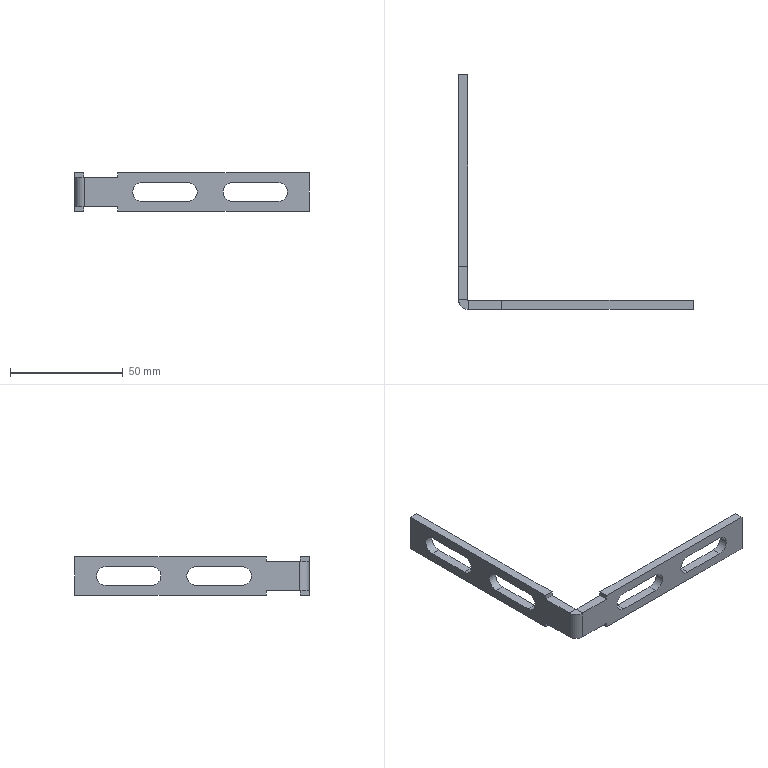Part | SolidWorks | features ICE 3, FlatPattern 1, SMBaseFlange 1, SheetMetal 1 | 1 solid | 40 faces | box 104 x 104 x 17 mm | volume 9651 mm3 | plane 28 | cylinder 12 | commonest cylinder face diameters 8.5 x10 0.4 x1 8.4 x1
STEP:
#1=CARTESIAN_POINT('',(4.,30.,12.75));
#2=VERTEX_POINT('',#1);
#3=CARTESIAN_POINT('',(4.,25.75,8.5));
#4=VERTEX_POINT('',#3);
#5=CARTESIAN_POINT('',(4.,30.,8.5));
#6=DIRECTION('',(1.,0.,0.));
#7=DIRECTION('',(0.,1.,0.));
#8=AXIS2_PLACEMENT_3D('',#5,#6,#7);
#9=CIRCLE('',#8,4.25);
#10=EDGE_CURVE('',#2,#4,#9,.T.);
#11=ORIENTED_EDGE('',*,*,#10,.T.);
#12=CARTESIAN_POINT('',(0.,25.75,8.5));
#13=VERTEX_POINT('',#12);
#14=CARTESIAN_POINT('',(10.,25.75,8.5));
#15=DIRECTION('',(-1.,0.,0.));
#16=VECTOR('',#15,1000.);
#17=LINE('',#14,#16);
#18=EDGE_CURVE('',#4,#13,#17,.T.);
#19=ORIENTED_EDGE('',*,*,#18,.T.);
#20=CARTESIAN_POINT('',(0.,30.,12.75));
#21=VERTEX_POINT('',#20);
#22=CARTESIAN_POINT('',(0.,30.,8.5));
#23=DIRECTION('',(-1.,0.,0.));
#24=DIRECTION('',(0.,-1.,0.));
#25=AXIS2_PLACEMENT_3D('',#22,#23,#24);
#26=CIRCLE('',#25,4.25);
#27=EDGE_CURVE('',#13,#21,#26,.T.);
#28=ORIENTED_EDGE('',*,*,#27,.T.);
#29=CARTESIAN_POINT('',(10.,30.,12.75));
#30=DIRECTION('',(-1.,0.,0.));
#31=VECTOR('',#30,1000.);
#32=LINE('',#29,#31);
#33=EDGE_CURVE('',#2,#21,#32,.T.);
#34=ORIENTED_EDGE('',*,*,#33,.F.);
#35=EDGE_LOOP('',(#11,#19,#28,#34));
#36=FACE_OUTER_BOUND('',#35,.T.);
#37=CARTESIAN_POINT('',(10.,30.,8.5));
#38=DIRECTION('',(-1.,0.,0.));
#39=DIRECTION('',(0.,-1.,0.));
#40=AXIS2_PLACEMENT_3D('',#37,#38,#39);
#41=CYLINDRICAL_SURFACE('',#40,4.25);
#42=ADVANCED_FACE('',(#36),#41,.F.);
#43=CARTESIAN_POINT('',(4.,70.,12.75));
#44=VERTEX_POINT('',#43);
#45=CARTESIAN_POINT('',(4.,65.75,8.5));
#46=VERTEX_POINT('',#45);
#47=CARTESIAN_POINT('',(4.,70.,8.5));
#48=DIRECTION('',(1.,0.,0.));
#49=DIRECTION('',(0.,1.,0.));
#50=AXIS2_PLACEMENT_3D('',#47,#48,#49);
#51=CIRCLE('',#50,4.25);
#52=EDGE_CURVE('',#44,#46,#51,.T.);
#53=ORIENTED_EDGE('',*,*,#52,.T.);
#54=CARTESIAN_POINT('',(0.,65.75,8.5));
#55=VERTEX_POINT('',#54);
#56=CARTESIAN_POINT('',(10.,65.75,8.5));
#57=DIRECTION('',(-1.,0.,0.));
#58=VECTOR('',#57,1000.);
#59=LINE('',#56,#58);
#60=EDGE_CURVE('',#46,#55,#59,.T.);
#61=ORIENTED_EDGE('',*,*,#60,.T.);
#62=CARTESIAN_POINT('',(0.,70.,12.75));
#63=VERTEX_POINT('',#62);
#64=CARTESIAN_POINT('',(0.,70.,8.5));
#65=DIRECTION('',(-1.,0.,0.));
#66=DIRECTION('',(0.,-1.,0.));
#67=AXIS2_PLACEMENT_3D('',#64,#65,#66);
#68=CIRCLE('',#67,4.25);
#69=EDGE_CURVE('',#55,#63,#68,.T.);
#70=ORIENTED_EDGE('',*,*,#69,.T.);
#71=CARTESIAN_POINT('',(10.,70.,12.75));
#72=DIRECTION('',(-1.,0.,0.));
#73=VECTOR('',#72,1000.);
#74=LINE('',#71,#73);
#75=EDGE_CURVE('',#44,#63,#74,.T.);
#76=ORIENTED_EDGE('',*,*,#75,.F.);
#77=EDGE_LOOP('',(#53,#61,#70,#76));
#78=FACE_OUTER_BOUND('',#77,.T.);
#79=CARTESIAN_POINT('',(10.,70.,8.5));
#80=DIRECTION('',(-1.,0.,0.));
#81=DIRECTION('',(0.,-1.,0.));
#82=AXIS2_PLACEMENT_3D('',#79,#80,#81);
#83=CYLINDRICAL_SURFACE('',#82,4.25);
#84=ADVANCED_FACE('',(#78),#83,.F.);
#85=CARTESIAN_POINT('',(0.,19.,15.));
#86=VERTEX_POINT('',#85);
#87=CARTESIAN_POINT('',(0.,4.2,15.));
#88=VERTEX_POINT('',#87);
#89=CARTESIAN_POINT('',(0.,0.,15.));
#90=DIRECTION('',(0.,-1.,0.));
#91=VECTOR('',#90,1000.);
#92=LINE('',#89,#91);
#93=EDGE_CURVE('',#86,#88,#92,.T.);
#94=ORIENTED_EDGE('',*,*,#93,.T.);
#95=CARTESIAN_POINT('',(4.,4.2,15.));
#96=VERTEX_POINT('',#95);
#97=CARTESIAN_POINT('',(0.,4.2,15.));
#98=DIRECTION('',(1.,0.,0.));
#99=VECTOR('',#98,1000.);
#100=LINE('',#97,#99);
#101=EDGE_CURVE('',#88,#96,#100,.T.);
#102=ORIENTED_EDGE('',*,*,#101,.T.);
#103=CARTESIAN_POINT('',(4.,19.,15.));
#104=VERTEX_POINT('',#103);
#105=CARTESIAN_POINT('',(4.,104.,15.));
#106=DIRECTION('',(0.,1.,0.));
#107=VECTOR('',#106,1000.);
#108=LINE('',#105,#107);
#109=EDGE_CURVE('',#96,#104,#108,.T.);
#110=ORIENTED_EDGE('',*,*,#109,.T.);
#111=CARTESIAN_POINT('',(19.,19.,15.));
#112=DIRECTION('',(-1.,0.,0.));
#113=VECTOR('',#112,1000.);
#114=LINE('',#111,#113);
#115=EDGE_CURVE('',#104,#86,#114,.T.);
#116=ORIENTED_EDGE('',*,*,#115,.T.);
#117=EDGE_LOOP('',(#94,#102,#110,#116));
#118=FACE_OUTER_BOUND('',#117,.T.);
#119=CARTESIAN_POINT('',(19.,0.,15.));
#120=DIRECTION('',(0.,0.,-1.));
#121=DIRECTION('',(-1.,0.,0.));
#122=AXIS2_PLACEMENT_3D('',#119,#120,#121);
#123=PLANE('',#122);
#124=ADVANCED_FACE('',(#118),#123,.F.);
#125=CARTESIAN_POINT('',(19.,4.,15.));
#126=VERTEX_POINT('',#125);
#127=CARTESIAN_POINT('',(4.2,4.,15.));
#128=VERTEX_POINT('',#127);
#129=CARTESIAN_POINT('',(0.,4.,15.));
#130=DIRECTION('',(-1.,0.,0.));
#131=VECTOR('',#130,1000.);
#132=LINE('',#129,#131);
#133=EDGE_CURVE('',#126,#128,#132,.T.);
#134=ORIENTED_EDGE('',*,*,#133,.T.);
#135=CARTESIAN_POINT('',(4.2,0.,15.));
#136=VERTEX_POINT('',#135);
#137=CARTESIAN_POINT('',(4.2,4.,15.));
#138=DIRECTION('',(0.,-1.,0.));
#139=VECTOR('',#138,1000.);
#140=LINE('',#137,#139);
#141=EDGE_CURVE('',#128,#136,#140,.T.);
#142=ORIENTED_EDGE('',*,*,#141,.T.);
#143=CARTESIAN_POINT('',(19.,0.,15.));
#144=VERTEX_POINT('',#143);
#145=CARTESIAN_POINT('',(19.,0.,15.));
#146=DIRECTION('',(-1.,0.,0.));
#147=VECTOR('',#146,1000.);
#148=LINE('',#145,#147);
#149=EDGE_CURVE('',#144,#136,#148,.T.);
#150=ORIENTED_EDGE('',*,*,#149,.F.);
#151=CARTESIAN_POINT('',(19.,0.,15.));
#152=DIRECTION('',(0.,-1.,0.));
#153=VECTOR('',#152,1000.);
#154=LINE('',#151,#153);
#155=EDGE_CURVE('',#126,#144,#154,.T.);
#156=ORIENTED_EDGE('',*,*,#155,.F.);
#157=EDGE_LOOP('',(#134,#142,#150,#156));
#158=FACE_OUTER_BOUND('',#157,.T.);
#159=CARTESIAN_POINT('',(19.,0.,15.));
#160=DIRECTION('',(0.,0.,-1.));
#161=DIRECTION('',(-1.,0.,0.));
#162=AXIS2_PLACEMENT_3D('',#159,#160,#161);
#163=PLANE('',#162);
#164=ADVANCED_FACE('',(#158),#163,.F.);
#165=CARTESIAN_POINT('',(4.,19.,2.));
#166=VERTEX_POINT('',#165);
#167=CARTESIAN_POINT('',(4.,4.2,2.));
#168=VERTEX_POINT('',#167);
#169=CARTESIAN_POINT('',(4.,104.,2.));
#170=DIRECTION('',(0.,-1.,0.));
#171=VECTOR('',#170,1000.);
#172=LINE('',#169,#171);
#173=EDGE_CURVE('',#166,#168,#172,.T.);
#174=ORIENTED_EDGE('',*,*,#173,.T.);
#175=CARTESIAN_POINT('',(0.,4.2,2.));
#176=VERTEX_POINT('',#175);
#177=CARTESIAN_POINT('',(4.,4.2,2.));
#178=DIRECTION('',(-1.,0.,0.));
#179=VECTOR('',#178,1000.);
#180=LINE('',#177,#179);
#181=EDGE_CURVE('',#168,#176,#180,.T.);
#182=ORIENTED_EDGE('',*,*,#181,.T.);
#183=CARTESIAN_POINT('',(0.,19.,2.));
#184=VERTEX_POINT('',#183);
#185=CARTESIAN_POINT('',(0.,0.,2.));
#186=DIRECTION('',(0.,1.,0.));
#187=VECTOR('',#186,1000.);
#188=LINE('',#185,#187);
#189=EDGE_CURVE('',#176,#184,#188,.T.);
#190=ORIENTED_EDGE('',*,*,#189,.T.);
#191=CARTESIAN_POINT('',(19.,19.,2.));
#192=DIRECTION('',(-1.,0.,0.));
#193=VECTOR('',#192,1000.);
#194=LINE('',#191,#193);
#195=EDGE_CURVE('',#166,#184,#194,.T.);
#196=ORIENTED_EDGE('',*,*,#195,.F.);
#197=EDGE_LOOP('',(#174,#182,#190,#196));
#198=FACE_OUTER_BOUND('',#197,.T.);
#199=CARTESIAN_POINT('',(19.,0.,2.));
#200=DIRECTION('',(0.,0.,1.));
#201=DIRECTION('',(1.,0.,0.));
#202=AXIS2_PLACEMENT_3D('',#199,#200,#201);
#203=PLANE('',#202);
#204=ADVANCED_FACE('',(#198),#203,.F.);
#205=CARTESIAN_POINT('',(19.,0.,2.));
#206=VERTEX_POINT('',#205);
#207=CARTESIAN_POINT('',(4.2,0.,2.));
#208=VERTEX_POINT('',#207);
#209=CARTESIAN_POINT('',(19.,0.,2.));
#210=DIRECTION('',(-1.,0.,0.));
#211=VECTOR('',#210,1000.);
#212=LINE('',#209,#211);
#213=EDGE_CURVE('',#206,#208,#212,.T.);
#214=ORIENTED_EDGE('',*,*,#213,.T.);
#215=CARTESIAN_POINT('',(4.2,4.,2.));
#216=VERTEX_POINT('',#215);
#217=CARTESIAN_POINT('',(4.2,0.,2.));
#218=DIRECTION('',(0.,1.,0.));
#219=VECTOR('',#218,1000.);
#220=LINE('',#217,#219);
#221=EDGE_CURVE('',#208,#216,#220,.T.);
#222=ORIENTED_EDGE('',*,*,#221,.T.);
#223=CARTESIAN_POINT('',(19.,4.,2.));
#224=VERTEX_POINT('',#223);
#225=CARTESIAN_POINT('',(0.,4.,2.));
#226=DIRECTION('',(1.,0.,0.));
#227=VECTOR('',#226,1000.);
#228=LINE('',#225,#227);
#229=EDGE_CURVE('',#216,#224,#228,.T.);
#230=ORIENTED_EDGE('',*,*,#229,.T.);
#231=CARTESIAN_POINT('',(19.,0.,2.));
#232=DIRECTION('',(0.,1.,0.));
#233=VECTOR('',#232,1000.);
#234=LINE('',#231,#233);
#235=EDGE_CURVE('',#206,#224,#234,.T.);
#236=ORIENTED_EDGE('',*,*,#235,.F.);
#237=EDGE_LOOP('',(#214,#222,#230,#236));
#238=FACE_OUTER_BOUND('',#237,.T.);
#239=CARTESIAN_POINT('',(19.,0.,2.));
#240=DIRECTION('',(0.,0.,1.));
#241=DIRECTION('',(1.,0.,0.));
#242=AXIS2_PLACEMENT_3D('',#239,#240,#241);
#243=PLANE('',#242);
#244=ADVANCED_FACE('',(#238),#243,.F.);
#245=CARTESIAN_POINT('',(19.,0.,0.));
#246=VERTEX_POINT('',#245);
#247=CARTESIAN_POINT('',(104.,0.,0.));
#248=VERTEX_POINT('',#247);
#249=CARTESIAN_POINT('',(0.,0.,0.));
#250=DIRECTION('',(1.,0.,0.));
#251=VECTOR('',#250,1000.);
#252=LINE('',#249,#251);
#253=EDGE_CURVE('',#246,#248,#252,.T.);
#254=ORIENTED_EDGE('',*,*,#253,.F.);
#255=CARTESIAN_POINT('',(19.,4.,0.));
#256=VERTEX_POINT('',#255);
#257=CARTESIAN_POINT('',(19.,0.,0.));
#258=DIRECTION('',(0.,-1.,0.));
#259=VECTOR('',#258,1000.);
#260=LINE('',#257,#259);
#261=EDGE_CURVE('',#256,#246,#260,.T.);
#262=ORIENTED_EDGE('',*,*,#261,.F.);
#263=CARTESIAN_POINT('',(104.,4.,0.));
#264=VERTEX_POINT('',#263);
#265=CARTESIAN_POINT('',(0.,4.,0.));
#266=DIRECTION('',(1.,0.,0.));
#267=VECTOR('',#266,1000.);
#268=LINE('',#265,#267);
#269=EDGE_CURVE('',#256,#264,#268,.T.);
#270=ORIENTED_EDGE('',*,*,#269,.T.);
#271=CARTESIAN_POINT('',(104.,4.,0.));
#272=DIRECTION('',(0.,-1.,0.));
#273=VECTOR('',#272,1000.);
#274=LINE('',#271,#273);
#275=EDGE_CURVE('',#264,#248,#274,.T.);
#276=ORIENTED_EDGE('',*,*,#275,.T.);
#277=EDGE_LOOP('',(#254,#262,#270,#276));
#278=FACE_OUTER_BOUND('',#277,.T.);
#279=CARTESIAN_POINT('',(4.,4.2,0.));
#280=DIRECTION('',(0.,0.,-1.));
#281=DIRECTION('',(-1.,0.,0.));
#282=AXIS2_PLACEMENT_3D('',#279,#280,#281);
#283=PLANE('',#282);
#284=ADVANCED_FACE('',(#278),#283,.T.);
#285=CARTESIAN_POINT('',(19.,4.,17.));
#286=VERTEX_POINT('',#285);
#287=CARTESIAN_POINT('',(104.,4.,17.));
#288=VERTEX_POINT('',#287);
#289=CARTESIAN_POINT('',(0.,4.,17.));
#290=DIRECTION('',(1.,0.,0.));
#291=VECTOR('',#290,1000.);
#292=LINE('',#289,#291);
#293=EDGE_CURVE('',#286,#288,#292,.T.);
#294=ORIENTED_EDGE('',*,*,#293,.F.);
#295=CARTESIAN_POINT('',(19.,0.,17.));
#296=VERTEX_POINT('',#295);
#297=CARTESIAN_POINT('',(19.,0.,17.));
#298=DIRECTION('',(0.,1.,0.));
#299=VECTOR('',#298,1000.);
#300=LINE('',#297,#299);
#301=EDGE_CURVE('',#296,#286,#300,.T.);
#302=ORIENTED_EDGE('',*,*,#301,.F.);
#303=CARTESIAN_POINT('',(104.,0.,17.));
#304=VERTEX_POINT('',#303);
#305=CARTESIAN_POINT('',(0.,0.,17.));
#306=DIRECTION('',(1.,0.,0.));
#307=VECTOR('',#306,1000.);
#308=LINE('',#305,#307);
#309=EDGE_CURVE('',#296,#304,#308,.T.);
#310=ORIENTED_EDGE('',*,*,#309,.T.);
#311=CARTESIAN_POINT('',(104.,4.,17.));
#312=DIRECTION('',(0.,-1.,0.));
#313=VECTOR('',#312,1000.);
#314=LINE('',#311,#313);
#315=EDGE_CURVE('',#288,#304,#314,.T.);
#316=ORIENTED_EDGE('',*,*,#315,.F.);
#317=EDGE_LOOP('',(#294,#302,#310,#316));
#318=FACE_OUTER_BOUND('',#317,.T.);
#319=CARTESIAN_POINT('',(4.2,4.2,17.));
#320=DIRECTION('',(0.,0.,1.));
#321=DIRECTION('',(1.,0.,0.));
#322=AXIS2_PLACEMENT_3D('',#319,#320,#321);
#323=PLANE('',#322);
#324=ADVANCED_FACE('',(#318),#323,.T.);
#325=CARTESIAN_POINT('',(4.,19.,17.));
#326=VERTEX_POINT('',#325);
#327=CARTESIAN_POINT('',(0.,19.,17.));
#328=VERTEX_POINT('',#327);
#329=CARTESIAN_POINT('',(19.,19.,17.));
#330=DIRECTION('',(-1.,0.,0.));
#331=VECTOR('',#330,1000.);
#332=LINE('',#329,#331);
#333=EDGE_CURVE('',#326,#328,#332,.T.);
#334=ORIENTED_EDGE('',*,*,#333,.F.);
#335=CARTESIAN_POINT('',(4.,104.,17.));
#336=VERTEX_POINT('',#335);
#337=CARTESIAN_POINT('',(4.,104.,17.));
#338=DIRECTION('',(0.,-1.,0.));
#339=VECTOR('',#338,1000.);
#340=LINE('',#337,#339);
#341=EDGE_CURVE('',#336,#326,#340,.T.);
#342=ORIENTED_EDGE('',*,*,#341,.F.);
#343=CARTESIAN_POINT('',(0.,104.,17.));
#344=VERTEX_POINT('',#343);
#345=CARTESIAN_POINT('',(0.,104.,17.));
#346=DIRECTION('',(1.,0.,0.));
#347=VECTOR('',#346,1000.);
#348=LINE('',#345,#347);
#349=EDGE_CURVE('',#344,#336,#348,.T.);
#350=ORIENTED_EDGE('',*,*,#349,.F.);
#351=CARTESIAN_POINT('',(0.,104.,17.));
#352=DIRECTION('',(0.,-1.,0.));
#353=VECTOR('',#352,1000.);
#354=LINE('',#351,#353);
#355=EDGE_CURVE('',#344,#328,#354,.T.);
#356=ORIENTED_EDGE('',*,*,#355,.T.);
#357=EDGE_LOOP('',(#334,#342,#350,#356));
#358=FACE_OUTER_BOUND('',#357,.T.);
#359=CARTESIAN_POINT('',(4.2,4.,17.));
#360=DIRECTION('',(0.,0.,1.));
#361=DIRECTION('',(1.,0.,0.));
#362=AXIS2_PLACEMENT_3D('',#359,#360,#361);
#363=PLANE('',#362);
#364=ADVANCED_FACE('',(#358),#363,.T.);
#365=CARTESIAN_POINT('',(30.,0.,4.25));
#366=VERTEX_POINT('',#365);
#367=CARTESIAN_POINT('',(50.,0.,4.25));
#368=VERTEX_POINT('',#367);
#369=CARTESIAN_POINT('',(30.,0.,4.25));
#370=DIRECTION('',(1.,0.,0.));
#371=VECTOR('',#370,1000.);
#372=LINE('',#369,#371);
#373=EDGE_CURVE('',#366,#368,#372,.T.);
#374=ORIENTED_EDGE('',*,*,#373,.F.);
#375=CARTESIAN_POINT('',(30.,0.,12.75));
#376=VERTEX_POINT('',#375);
#377=CARTESIAN_POINT('',(30.,0.,8.5));
#378=DIRECTION('',(0.,-1.,0.));
#379=DIRECTION('',(0.,0.,-1.));
#380=AXIS2_PLACEMENT_3D('',#377,#378,#379);
#381=CIRCLE('',#380,4.25);
#382=EDGE_CURVE('',#376,#366,#381,.T.);
#383=ORIENTED_EDGE('',*,*,#382,.F.);
#384=CARTESIAN_POINT('',(50.,0.,12.75));
#385=VERTEX_POINT('',#384);
#386=CARTESIAN_POINT('',(30.,0.,12.75));
#387=DIRECTION('',(-1.,0.,0.));
#388=VECTOR('',#387,1000.);
#389=LINE('',#386,#388);
#390=EDGE_CURVE('',#385,#376,#389,.T.);
#391=ORIENTED_EDGE('',*,*,#390,.F.);
#392=CARTESIAN_POINT('',(50.,0.,8.5));
#393=DIRECTION('',(0.,-1.,0.));
#394=DIRECTION('',(0.,0.,-1.));
#395=AXIS2_PLACEMENT_3D('',#392,#393,#394);
#396=CIRCLE('',#395,4.25);
#397=EDGE_CURVE('',#368,#385,#396,.T.);
#398=ORIENTED_EDGE('',*,*,#397,.F.);
#399=EDGE_LOOP('',(#374,#383,#391,#398));
#400=FACE_BOUND('',#399,.T.);
#401=CARTESIAN_POINT('',(70.,0.,4.25));
#402=VERTEX_POINT('',#401);
#403=CARTESIAN_POINT('',(90.,0.,4.25));
#404=VERTEX_POINT('',#403);
#405=CARTESIAN_POINT('',(70.,0.,4.25));
#406=DIRECTION('',(1.,0.,0.));
#407=VECTOR('',#406,1000.);
#408=LINE('',#405,#407);
#409=EDGE_CURVE('',#402,#404,#408,.T.);
#410=ORIENTED_EDGE('',*,*,#409,.F.);
#411=CARTESIAN_POINT('',(70.,0.,12.75));
#412=VERTEX_POINT('',#411);
#413=CARTESIAN_POINT('',(70.,0.,8.5));
#414=DIRECTION('',(0.,-1.,0.));
#415=DIRECTION('',(0.,0.,-1.));
#416=AXIS2_PLACEMENT_3D('',#413,#414,#415);
#417=CIRCLE('',#416,4.25);
#418=EDGE_CURVE('',#412,#402,#417,.T.);
#419=ORIENTED_EDGE('',*,*,#418,.F.);
#420=CARTESIAN_POINT('',(90.,0.,12.75));
#421=VERTEX_POINT('',#420);
#422=CARTESIAN_POINT('',(70.,0.,12.75));
#423=DIRECTION('',(-1.,0.,0.));
#424=VECTOR('',#423,1000.);
#425=LINE('',#422,#424);
#426=EDGE_CURVE('',#421,#412,#425,.T.);
#427=ORIENTED_EDGE('',*,*,#426,.F.);
#428=CARTESIAN_POINT('',(90.,0.,8.5));
#429=DIRECTION('',(0.,-1.,0.));
#430=DIRECTION('',(0.,0.,-1.));
#431=AXIS2_PLACEMENT_3D('',#428,#429,#430);
#432=CIRCLE('',#431,4.25);
#433=EDGE_CURVE('',#404,#421,#432,.T.);
#434=ORIENTED_EDGE('',*,*,#433,.F.);
#435=EDGE_LOOP('',(#410,#419,#427,#434));
#436=FACE_BOUND('',#435,.T.);
#437=CARTESIAN_POINT('',(19.,0.,17.));
#438=DIRECTION('',(0.,0.,1.));
#439=VECTOR('',#438,1000.);
#440=LINE('',#437,#439);
#441=EDGE_CURVE('',#144,#296,#440,.T.);
#442=ORIENTED_EDGE('',*,*,#441,.F.);
#443=ORIENTED_EDGE('',*,*,#149,.T.);
#444=CARTESIAN_POINT('',(4.2,0.,17.));
#445=DIRECTION('',(0.,0.,-1.));
#446=VECTOR('',#445,1000.);
#447=LINE('',#444,#446);
#448=EDGE_CURVE('',#136,#208,#447,.T.);
#449=ORIENTED_EDGE('',*,*,#448,.T.);
#450=ORIENTED_EDGE('',*,*,#213,.F.);
#451=CARTESIAN_POINT('',(19.,0.,0.));
#452=DIRECTION('',(0.,0.,1.));
#453=VECTOR('',#452,1000.);
#454=LINE('',#451,#453);
#455=EDGE_CURVE('',#246,#206,#454,.T.);
#456=ORIENTED_EDGE('',*,*,#455,.F.);
#457=ORIENTED_EDGE('',*,*,#253,.T.);
#458=CARTESIAN_POINT('',(104.,0.,17.));
#459=DIRECTION('',(0.,0.,-1.));
#460=VECTOR('',#459,1000.);
#461=LINE('',#458,#460);
#462=EDGE_CURVE('',#304,#248,#461,.T.);
#463=ORIENTED_EDGE('',*,*,#462,.F.);
#464=ORIENTED_EDGE('',*,*,#309,.F.);
#465=EDGE_LOOP('',(#442,#443,#449,#450,#456,#457,#463,#464));
#466=FACE_OUTER_BOUND('',#465,.T.);
#467=CARTESIAN_POINT('',(0.,0.,17.));
#468=DIRECTION('',(0.,1.,0.));
#469=DIRECTION('',(0.,0.,1.));
#470=AXIS2_PLACEMENT_3D('',#467,#468,#469);
#471=PLANE('',#470);
#472=ADVANCED_FACE('',(#400,#436,#466),#471,.F.);
#473=ORIENTED_EDGE('',*,*,#275,.F.);
#474=CARTESIAN_POINT('',(104.,4.,17.));
#475=DIRECTION('',(0.,0.,-1.));
#476=VECTOR('',#475,1000.);
#477=LINE('',#474,#476);
#478=EDGE_CURVE('',#288,#264,#477,.T.);
#479=ORIENTED_EDGE('',*,*,#478,.F.);
#480=ORIENTED_EDGE('',*,*,#315,.T.);
#481=ORIENTED_EDGE('',*,*,#462,.T.);
#482=EDGE_LOOP('',(#473,#479,#480,#481));
#483=FACE_OUTER_BOUND('',#482,.T.);
#484=CARTESIAN_POINT('',(104.,4.,17.));
#485=DIRECTION('',(1.,0.,0.));
#486=DIRECTION('',(0.,0.,-1.));
#487=AXIS2_PLACEMENT_3D('',#484,#485,#486);
#488=PLANE('',#487);
#489=ADVANCED_FACE('',(#483),#488,.T.);
#490=ORIENTED_EDGE('',*,*,#133,.F.);
#491=CARTESIAN_POINT('',(19.,4.,17.));
#492=DIRECTION('',(0.,0.,1.));
#493=VECTOR('',#492,1000.);
#494=LINE('',#491,#493);
#495=EDGE_CURVE('',#126,#286,#494,.T.);
#496=ORIENTED_EDGE('',*,*,#495,.T.);
#497=ORIENTED_EDGE('',*,*,#293,.T.);
#498=ORIENTED_EDGE('',*,*,#478,.T.);
#499=ORIENTED_EDGE('',*,*,#269,.F.);
#500=CARTESIAN_POINT('',(19.,4.,17.));
#501=DIRECTION('',(0.,0.,1.));
#502=VECTOR('',#501,1000.);
#503=LINE('',#500,#502);
#504=EDGE_CURVE('',#256,#224,#503,.T.);
#505=ORIENTED_EDGE('',*,*,#504,.T.);
#506=ORIENTED_EDGE('',*,*,#229,.F.);
#507=CARTESIAN_POINT('',(4.2,4.,17.));
#508=DIRECTION('',(0.,0.,-1.));
#509=VECTOR('',#508,1000.);
#510=LINE('',#507,#509);
#511=EDGE_CURVE('',#128,#216,#510,.T.);
#512=ORIENTED_EDGE('',*,*,#511,.F.);
#513=EDGE_LOOP('',(#490,#496,#497,#498,#499,#505,#506,#512));
#514=FACE_OUTER_BOUND('',#513,.T.);
#515=CARTESIAN_POINT('',(30.,4.,4.25));
#516=VERTEX_POINT('',#515);
#517=CARTESIAN_POINT('',(30.,4.,12.75));
#518=VERTEX_POINT('',#517);
#519=CARTESIAN_POINT('',(30.,4.,8.5));
#520=DIRECTION('',(0.,1.,0.));
#521=DIRECTION('',(0.,0.,1.));
#522=AXIS2_PLACEMENT_3D('',#519,#520,#521);
#523=CIRCLE('',#522,4.25);
#524=EDGE_CURVE('',#516,#518,#523,.T.);
#525=ORIENTED_EDGE('',*,*,#524,.F.);
#526=CARTESIAN_POINT('',(50.,4.,4.25));
#527=VERTEX_POINT('',#526);
#528=CARTESIAN_POINT('',(0.,4.,4.25));
#529=DIRECTION('',(-1.,0.,0.));
#530=VECTOR('',#529,1000.);
#531=LINE('',#528,#530);
#532=EDGE_CURVE('',#527,#516,#531,.T.);
#533=ORIENTED_EDGE('',*,*,#532,.F.);
#534=CARTESIAN_POINT('',(50.,4.,12.75));
#535=VERTEX_POINT('',#534);
#536=CARTESIAN_POINT('',(50.,4.,8.5));
#537=DIRECTION('',(0.,1.,0.));
#538=DIRECTION('',(0.,0.,1.));
#539=AXIS2_PLACEMENT_3D('',#536,#537,#538);
#540=CIRCLE('',#539,4.25);
#541=EDGE_CURVE('',#535,#527,#540,.T.);
#542=ORIENTED_EDGE('',*,*,#541,.F.);
#543=CARTESIAN_POINT('',(0.,4.,12.75));
#544=DIRECTION('',(1.,0.,0.));
#545=VECTOR('',#544,1000.);
#546=LINE('',#543,#545);
#547=EDGE_CURVE('',#518,#535,#546,.T.);
#548=ORIENTED_EDGE('',*,*,#547,.F.);
#549=EDGE_LOOP('',(#525,#533,#542,#548));
#550=FACE_BOUND('',#549,.T.);
#551=CARTESIAN_POINT('',(70.,4.,4.25));
#552=VERTEX_POINT('',#551);
#553=CARTESIAN_POINT('',(70.,4.,12.75));
#554=VERTEX_POINT('',#553);
#555=CARTESIAN_POINT('',(70.,4.,8.5));
#556=DIRECTION('',(0.,1.,0.));
#557=DIRECTION('',(0.,0.,1.));
#558=AXIS2_PLACEMENT_3D('',#555,#556,#557);
#559=CIRCLE('',#558,4.25);
#560=EDGE_CURVE('',#552,#554,#559,.T.);
#561=ORIENTED_EDGE('',*,*,#560,.F.);
#562=CARTESIAN_POINT('',(90.,4.,4.25));
#563=VERTEX_POINT('',#562);
#564=CARTESIAN_POINT('',(0.,4.,4.25));
#565=DIRECTION('',(-1.,0.,0.));
#566=VECTOR('',#565,1000.);
#567=LINE('',#564,#566);
#568=EDGE_CURVE('',#563,#552,#567,.T.);
#569=ORIENTED_EDGE('',*,*,#568,.F.);
#570=CARTESIAN_POINT('',(90.,4.,12.75));
#571=VERTEX_POINT('',#570);
#572=CARTESIAN_POINT('',(90.,4.,8.5));
#573=DIRECTION('',(0.,1.,0.));
#574=DIRECTION('',(0.,0.,1.));
#575=AXIS2_PLACEMENT_3D('',#572,#573,#574);
#576=CIRCLE('',#575,4.25);
#577=EDGE_CURVE('',#571,#563,#576,.T.);
#578=ORIENTED_EDGE('',*,*,#577,.F.);
#579=CARTESIAN_POINT('',(0.,4.,12.75));
#580=DIRECTION('',(1.,0.,0.));
#581=VECTOR('',#580,1000.);
#582=LINE('',#579,#581);
#583=EDGE_CURVE('',#554,#571,#582,.T.);
#584=ORIENTED_EDGE('',*,*,#583,.F.);
#585=EDGE_LOOP('',(#561,#569,#578,#584));
#586=FACE_BOUND('',#585,.T.);
#587=CARTESIAN_POINT('',(0.,4.,17.));
#588=DIRECTION('',(0.,1.,0.));
#589=DIRECTION('',(0.,0.,1.));
#590=AXIS2_PLACEMENT_3D('',#587,#588,#589);
#591=PLANE('',#590);
#592=ADVANCED_FACE('',(#514,#550,#586),#591,.T.);
#593=CARTESIAN_POINT('',(4.2,4.2,15.));
#594=DIRECTION('',(0.,0.,-1.));
#595=DIRECTION('',(-1.,0.,0.));
#596=AXIS2_PLACEMENT_3D('',#593,#594,#595);
#597=CIRCLE('',#596,0.2);
#598=EDGE_CURVE('',#128,#96,#597,.T.);
#599=ORIENTED_EDGE('',*,*,#598,.F.);
#600=ORIENTED_EDGE('',*,*,#511,.T.);
#601=CARTESIAN_POINT('',(4.2,4.2,2.));
#602=DIRECTION('',(0.,0.,1.));
#603=DIRECTION('',(1.,0.,0.));
#604=AXIS2_PLACEMENT_3D('',#601,#602,#603);
#605=CIRCLE('',#604,0.2);
#606=EDGE_CURVE('',#168,#216,#605,.T.);
#607=ORIENTED_EDGE('',*,*,#606,.F.);
#608=CARTESIAN_POINT('',(4.,4.2,17.));
#609=DIRECTION('',(0.,0.,-1.));
#610=VECTOR('',#609,1000.);
#611=LINE('',#608,#610);
#612=EDGE_CURVE('',#96,#168,#611,.T.);
#613=ORIENTED_EDGE('',*,*,#612,.F.);
#614=EDGE_LOOP('',(#599,#600,#607,#613));
#615=FACE_OUTER_BOUND('',#614,.T.);
#616=CARTESIAN_POINT('',(4.2,4.2,17.));
#617=DIRECTION('',(0.,0.,-1.));
#618=DIRECTION('',(-1.,0.,0.));
#619=AXIS2_PLACEMENT_3D('',#616,#617,#618);
#620=CYLINDRICAL_SURFACE('',#619,0.2);
#621=ADVANCED_FACE('',(#615),#620,.F.);
#622=ORIENTED_EDGE('',*,*,#109,.F.);
#623=ORIENTED_EDGE('',*,*,#612,.T.);
#624=ORIENTED_EDGE('',*,*,#173,.F.);
#625=CARTESIAN_POINT('',(4.,19.,0.));
#626=VERTEX_POINT('',#625);
#627=CARTESIAN_POINT('',(4.,19.,17.));
#628=DIRECTION('',(0.,0.,1.));
#629=VECTOR('',#628,1000.);
#630=LINE('',#627,#629);
#631=EDGE_CURVE('',#626,#166,#630,.T.);
#632=ORIENTED_EDGE('',*,*,#631,.F.);
#633=CARTESIAN_POINT('',(4.,104.,0.));
#634=VERTEX_POINT('',#633);
#635=CARTESIAN_POINT('',(4.,104.,0.));
#636=DIRECTION('',(0.,-1.,0.));
#637=VECTOR('',#636,1000.);
#638=LINE('',#635,#637);
#639=EDGE_CURVE('',#634,#626,#638,.T.);
#640=ORIENTED_EDGE('',*,*,#639,.F.);
#641=CARTESIAN_POINT('',(4.,104.,17.));
#642=DIRECTION('',(0.,0.,-1.));
#643=VECTOR('',#642,1000.);
#644=LINE('',#641,#643);
#645=EDGE_CURVE('',#336,#634,#644,.T.);
#646=ORIENTED_EDGE('',*,*,#645,.F.);
#647=ORIENTED_EDGE('',*,*,#341,.T.);
#648=CARTESIAN_POINT('',(4.,19.,17.));
#649=DIRECTION('',(0.,0.,1.));
#650=VECTOR('',#649,1000.);
#651=LINE('',#648,#650);
#652=EDGE_CURVE('',#104,#326,#651,.T.);
#653=ORIENTED_EDGE('',*,*,#652,.F.);
#654=EDGE_LOOP('',(#622,#623,#624,#632,#640,#646,#647,#653));
#655=FACE_OUTER_BOUND('',#654,.T.);
#656=CARTESIAN_POINT('',(4.,50.,4.25));
#657=VERTEX_POINT('',#656);
#658=CARTESIAN_POINT('',(4.,50.,12.75));
#659=VERTEX_POINT('',#658);
#660=CARTESIAN_POINT('',(4.,50.,8.5));
#661=DIRECTION('',(1.,0.,0.));
#662=DIRECTION('',(0.,1.,0.));
#663=AXIS2_PLACEMENT_3D('',#660,#661,#662);
#664=CIRCLE('',#663,4.25);
#665=EDGE_CURVE('',#657,#659,#664,.T.);
#666=ORIENTED_EDGE('',*,*,#665,.F.);
#667=CARTESIAN_POINT('',(4.,30.,4.25));
#668=VERTEX_POINT('',#667);
#669=CARTESIAN_POINT('',(4.,104.,4.25));
#670=DIRECTION('',(0.,1.,0.));
#671=VECTOR('',#670,1000.);
#672=LINE('',#669,#671);
#673=EDGE_CURVE('',#668,#657,#672,.T.);
#674=ORIENTED_EDGE('',*,*,#673,.F.);
#675=CARTESIAN_POINT('',(4.,30.,8.5));
#676=DIRECTION('',(1.,0.,0.));
#677=DIRECTION('',(0.,1.,0.));
#678=AXIS2_PLACEMENT_3D('',#675,#676,#677);
#679=CIRCLE('',#678,4.25);
#680=EDGE_CURVE('',#4,#668,#679,.T.);
#681=ORIENTED_EDGE('',*,*,#680,.F.);
#682=ORIENTED_EDGE('',*,*,#10,.F.);
#683=CARTESIAN_POINT('',(4.,104.,12.75));
#684=DIRECTION('',(0.,-1.,0.));
#685=VECTOR('',#684,1000.);
#686=LINE('',#683,#685);
#687=EDGE_CURVE('',#659,#2,#686,.T.);
#688=ORIENTED_EDGE('',*,*,#687,.F.);
#689=EDGE_LOOP('',(#666,#674,#681,#682,#688));
#690=FACE_BOUND('',#689,.T.);
#691=CARTESIAN_POINT('',(4.,90.,4.25));
#692=VERTEX_POINT('',#691);
#693=CARTESIAN_POINT('',(4.,90.,12.75));
#694=VERTEX_POINT('',#693);
#695=CARTESIAN_POINT('',(4.,90.,8.5));
#696=DIRECTION('',(1.,0.,0.));
#697=DIRECTION('',(0.,1.,0.));
#698=AXIS2_PLACEMENT_3D('',#695,#696,#697);
#699=CIRCLE('',#698,4.25);
#700=EDGE_CURVE('',#692,#694,#699,.T.);
#701=ORIENTED_EDGE('',*,*,#700,.F.);
#702=CARTESIAN_POINT('',(4.,70.,4.25));
#703=VERTEX_POINT('',#702);
#704=CARTESIAN_POINT('',(4.,104.,4.25));
#705=DIRECTION('',(0.,1.,0.));
#706=VECTOR('',#705,1000.);
#707=LINE('',#704,#706);
#708=EDGE_CURVE('',#703,#692,#707,.T.);
#709=ORIENTED_EDGE('',*,*,#708,.F.);
#710=CARTESIAN_POINT('',(4.,70.,8.5));
#711=DIRECTION('',(1.,0.,0.));
#712=DIRECTION('',(0.,1.,0.));
#713=AXIS2_PLACEMENT_3D('',#710,#711,#712);
#714=CIRCLE('',#713,4.25);
#715=EDGE_CURVE('',#46,#703,#714,.T.);
#716=ORIENTED_EDGE('',*,*,#715,.F.);
#717=ORIENTED_EDGE('',*,*,#52,.F.);
#718=CARTESIAN_POINT('',(4.,104.,12.75));
#719=DIRECTION('',(0.,-1.,0.));
#720=VECTOR('',#719,1000.);
#721=LINE('',#718,#720);
#722=EDGE_CURVE('',#694,#44,#721,.T.);
#723=ORIENTED_EDGE('',*,*,#722,.F.);
#724=EDGE_LOOP('',(#701,#709,#716,#717,#723));
#725=FACE_BOUND('',#724,.T.);
#726=CARTESIAN_POINT('',(4.,104.,17.));
#727=DIRECTION('',(1.,0.,0.));
#728=DIRECTION('',(0.,1.,0.));
#729=AXIS2_PLACEMENT_3D('',#726,#727,#728);
#730=PLANE('',#729);
#731=ADVANCED_FACE('',(#655,#690,#725),#730,.T.);
#732=CARTESIAN_POINT('',(0.,104.,0.));
#733=VERTEX_POINT('',#732);
#734=CARTESIAN_POINT('',(0.,104.,0.));
#735=DIRECTION('',(1.,0.,0.));
#736=VECTOR('',#735,1000.);
#737=LINE('',#734,#736);
#738=EDGE_CURVE('',#733,#634,#737,.T.);
#739=ORIENTED_EDGE('',*,*,#738,.F.);
#740=CARTESIAN_POINT('',(0.,104.,17.));
#741=DIRECTION('',(0.,0.,-1.));
#742=VECTOR('',#741,1000.);
#743=LINE('',#740,#742);
#744=EDGE_CURVE('',#344,#733,#743,.T.);
#745=ORIENTED_EDGE('',*,*,#744,.F.);
#746=ORIENTED_EDGE('',*,*,#349,.T.);
#747=ORIENTED_EDGE('',*,*,#645,.T.);
#748=EDGE_LOOP('',(#739,#745,#746,#747));
#749=FACE_OUTER_BOUND('',#748,.T.);
#750=CARTESIAN_POINT('',(0.,104.,17.));
#751=DIRECTION('',(0.,1.,0.));
#752=DIRECTION('',(0.,0.,1.));
#753=AXIS2_PLACEMENT_3D('',#750,#751,#752);
#754=PLANE('',#753);
#755=ADVANCED_FACE('',(#749),#754,.T.);
#756=CARTESIAN_POINT('',(0.,50.,4.25));
#757=VERTEX_POINT('',#756);
#758=CARTESIAN_POINT('',(0.,30.,4.25));
#759=VERTEX_POINT('',#758);
#760=CARTESIAN_POINT('',(0.,50.,4.25));
#761=DIRECTION('',(0.,-1.,0.));
#762=VECTOR('',#761,1000.);
#763=LINE('',#760,#762);
#764=EDGE_CURVE('',#757,#759,#763,.T.);
#765=ORIENTED_EDGE('',*,*,#764,.F.);
#766=CARTESIAN_POINT('',(0.,50.,12.75));
#767=VERTEX_POINT('',#766);
#768=CARTESIAN_POINT('',(0.,50.,8.5));
#769=DIRECTION('',(-1.,0.,0.));
#770=DIRECTION('',(0.,-1.,0.));
#771=AXIS2_PLACEMENT_3D('',#768,#769,#770);
#772=CIRCLE('',#771,4.25);
#773=EDGE_CURVE('',#767,#757,#772,.T.);
#774=ORIENTED_EDGE('',*,*,#773,.F.);
#775=CARTESIAN_POINT('',(0.,50.,12.75));
#776=DIRECTION('',(0.,1.,0.));
#777=VECTOR('',#776,1000.);
#778=LINE('',#775,#777);
#779=EDGE_CURVE('',#21,#767,#778,.T.);
#780=ORIENTED_EDGE('',*,*,#779,.F.);
#781=ORIENTED_EDGE('',*,*,#27,.F.);
#782=CARTESIAN_POINT('',(0.,30.,8.5));
#783=DIRECTION('',(-1.,0.,0.));
#784=DIRECTION('',(0.,-1.,0.));
#785=AXIS2_PLACEMENT_3D('',#782,#783,#784);
#786=CIRCLE('',#785,4.25);
#787=EDGE_CURVE('',#759,#13,#786,.T.);
#788=ORIENTED_EDGE('',*,*,#787,.F.);
#789=EDGE_LOOP('',(#765,#774,#780,#781,#788));
#790=FACE_BOUND('',#789,.T.);
#791=CARTESIAN_POINT('',(0.,90.,4.25));
#792=VERTEX_POINT('',#791);
#793=CARTESIAN_POINT('',(0.,70.,4.25));
#794=VERTEX_POINT('',#793);
#795=CARTESIAN_POINT('',(0.,90.,4.25));
#796=DIRECTION('',(0.,-1.,0.));
#797=VECTOR('',#796,1000.);
#798=LINE('',#795,#797);
#799=EDGE_CURVE('',#792,#794,#798,.T.);
#800=ORIENTED_EDGE('',*,*,#799,.F.);
#801=CARTESIAN_POINT('',(0.,90.,12.75));
#802=VERTEX_POINT('',#801);
#803=CARTESIAN_POINT('',(0.,90.,8.5));
#804=DIRECTION('',(-1.,0.,0.));
#805=DIRECTION('',(0.,-1.,0.));
#806=AXIS2_PLACEMENT_3D('',#803,#804,#805);
#807=CIRCLE('',#806,4.25);
#808=EDGE_CURVE('',#802,#792,#807,.T.);
#809=ORIENTED_EDGE('',*,*,#808,.F.);
#810=CARTESIAN_POINT('',(0.,90.,12.75));
#811=DIRECTION('',(0.,1.,0.));
#812=VECTOR('',#811,1000.);
#813=LINE('',#810,#812);
#814=EDGE_CURVE('',#63,#802,#813,.T.);
#815=ORIENTED_EDGE('',*,*,#814,.F.);
#816=ORIENTED_EDGE('',*,*,#69,.F.);
#817=CARTESIAN_POINT('',(0.,70.,8.5));
#818=DIRECTION('',(-1.,0.,0.));
#819=DIRECTION('',(0.,-1.,0.));
#820=AXIS2_PLACEMENT_3D('',#817,#818,#819);
#821=CIRCLE('',#820,4.25);
#822=EDGE_CURVE('',#794,#55,#821,.T.);
#823=ORIENTED_EDGE('',*,*,#822,.F.);
#824=EDGE_LOOP('',(#800,#809,#815,#816,#823));
#825=FACE_BOUND('',#824,.T.);
#826=CARTESIAN_POINT('',(0.,4.2,17.));
#827=DIRECTION('',(0.,0.,-1.));
#828=VECTOR('',#827,1000.);
#829=LINE('',#826,#828);
#830=EDGE_CURVE('',#88,#176,#829,.T.);
#831=ORIENTED_EDGE('',*,*,#830,.F.);
#832=ORIENTED_EDGE('',*,*,#93,.F.);
#833=CARTESIAN_POINT('',(0.,19.,17.));
#834=DIRECTION('',(0.,0.,-1.));
#835=VECTOR('',#834,1000.);
#836=LINE('',#833,#835);
#837=EDGE_CURVE('',#328,#86,#836,.T.);
#838=ORIENTED_EDGE('',*,*,#837,.F.);
#839=ORIENTED_EDGE('',*,*,#355,.F.);
#840=ORIENTED_EDGE('',*,*,#744,.T.);
#841=CARTESIAN_POINT('',(0.,19.,0.));
#842=VERTEX_POINT('',#841);
#843=CARTESIAN_POINT('',(0.,104.,0.));
#844=DIRECTION('',(0.,-1.,0.));
#845=VECTOR('',#844,1000.);
#846=LINE('',#843,#845);
#847=EDGE_CURVE('',#733,#842,#846,.T.);
#848=ORIENTED_EDGE('',*,*,#847,.T.);
#849=CARTESIAN_POINT('',(0.,19.,0.));
#850=DIRECTION('',(0.,0.,-1.));
#851=VECTOR('',#850,1000.);
#852=LINE('',#849,#851);
#853=EDGE_CURVE('',#184,#842,#852,.T.);
#854=ORIENTED_EDGE('',*,*,#853,.F.);
#855=ORIENTED_EDGE('',*,*,#189,.F.);
#856=EDGE_LOOP('',(#831,#832,#838,#839,#840,#848,#854,#855));
#857=FACE_OUTER_BOUND('',#856,.T.);
#858=CARTESIAN_POINT('',(0.,104.,17.));
#859=DIRECTION('',(1.,0.,0.));
#860=DIRECTION('',(0.,1.,0.));
#861=AXIS2_PLACEMENT_3D('',#858,#859,#860);
#862=PLANE('',#861);
#863=ADVANCED_FACE('',(#790,#825,#857),#862,.F.);
#864=ORIENTED_EDGE('',*,*,#448,.F.);
#865=CARTESIAN_POINT('',(4.2,4.2,15.));
#866=DIRECTION('',(0.,0.,-1.));
#867=DIRECTION('',(-1.,0.,0.));
#868=AXIS2_PLACEMENT_3D('',#865,#866,#867);
#869=CIRCLE('',#868,4.2);
#870=EDGE_CURVE('',#136,#88,#869,.T.);
#871=ORIENTED_EDGE('',*,*,#870,.T.);
#872=ORIENTED_EDGE('',*,*,#830,.T.);
#873=CARTESIAN_POINT('',(4.2,4.2,2.));
#874=DIRECTION('',(0.,0.,1.));
#875=DIRECTION('',(1.,0.,0.));
#876=AXIS2_PLACEMENT_3D('',#873,#874,#875);
#877=CIRCLE('',#876,4.2);
#878=EDGE_CURVE('',#176,#208,#877,.T.);
#879=ORIENTED_EDGE('',*,*,#878,.T.);
#880=EDGE_LOOP('',(#864,#871,#872,#879));
#881=FACE_OUTER_BOUND('',#880,.T.);
#882=CARTESIAN_POINT('',(4.2,4.2,17.));
#883=DIRECTION('',(0.,0.,-1.));
#884=DIRECTION('',(-1.,0.,0.));
#885=AXIS2_PLACEMENT_3D('',#882,#883,#884);
#886=CYLINDRICAL_SURFACE('',#885,4.2);
#887=ADVANCED_FACE('',(#881),#886,.T.);
#888=ORIENTED_EDGE('',*,*,#639,.T.);
#889=CARTESIAN_POINT('',(4.2,19.,0.));
#890=DIRECTION('',(-1.,0.,0.));
#891=VECTOR('',#890,1000.);
#892=LINE('',#889,#891);
#893=EDGE_CURVE('',#626,#842,#892,.T.);
#894=ORIENTED_EDGE('',*,*,#893,.T.);
#895=ORIENTED_EDGE('',*,*,#847,.F.);
#896=ORIENTED_EDGE('',*,*,#738,.T.);
#897=EDGE_LOOP('',(#888,#894,#895,#896));
#898=FACE_OUTER_BOUND('',#897,.T.);
#899=CARTESIAN_POINT('',(4.2,4.2,0.));
#900=DIRECTION('',(0.,0.,1.));
#901=DIRECTION('',(1.,0.,0.));
#902=AXIS2_PLACEMENT_3D('',#899,#900,#901);
#903=PLANE('',#902);
#904=ADVANCED_FACE('',(#898),#903,.F.);
#905=ORIENTED_EDGE('',*,*,#560,.T.);
#906=CARTESIAN_POINT('',(70.,10.,12.75));
#907=DIRECTION('',(0.,-1.,0.));
#908=VECTOR('',#907,1000.);
#909=LINE('',#906,#908);
#910=EDGE_CURVE('',#554,#412,#909,.T.);
#911=ORIENTED_EDGE('',*,*,#910,.T.);
#912=ORIENTED_EDGE('',*,*,#418,.T.);
#913=CARTESIAN_POINT('',(70.,10.,4.25));
#914=DIRECTION('',(0.,-1.,0.));
#915=VECTOR('',#914,1000.);
#916=LINE('',#913,#915);
#917=EDGE_CURVE('',#552,#402,#916,.T.);
#918=ORIENTED_EDGE('',*,*,#917,.F.);
#919=EDGE_LOOP('',(#905,#911,#912,#918));
#920=FACE_OUTER_BOUND('',#919,.T.);
#921=CARTESIAN_POINT('',(70.,10.,8.5));
#922=DIRECTION('',(0.,-1.,0.));
#923=DIRECTION('',(0.,0.,-1.));
#924=AXIS2_PLACEMENT_3D('',#921,#922,#923);
#925=CYLINDRICAL_SURFACE('',#924,4.25);
#926=ADVANCED_FACE('',(#920),#925,.F.);
#927=ORIENTED_EDGE('',*,*,#583,.T.);
#928=CARTESIAN_POINT('',(90.,10.,12.75));
#929=DIRECTION('',(0.,-1.,0.));
#930=VECTOR('',#929,1000.);
#931=LINE('',#928,#930);
#932=EDGE_CURVE('',#571,#421,#931,.T.);
#933=ORIENTED_EDGE('',*,*,#932,.T.);
#934=ORIENTED_EDGE('',*,*,#426,.T.);
#935=ORIENTED_EDGE('',*,*,#910,.F.);
#936=EDGE_LOOP('',(#927,#933,#934,#935));
#937=FACE_OUTER_BOUND('',#936,.T.);
#938=CARTESIAN_POINT('',(70.,10.,12.75));
#939=DIRECTION('',(0.,0.,1.));
#940=DIRECTION('',(1.,0.,0.));
#941=AXIS2_PLACEMENT_3D('',#938,#939,#940);
#942=PLANE('',#941);
#943=ADVANCED_FACE('',(#937),#942,.F.);
#944=ORIENTED_EDGE('',*,*,#577,.T.);
#945=CARTESIAN_POINT('',(90.,10.,4.25));
#946=DIRECTION('',(0.,-1.,0.));
#947=VECTOR('',#946,1000.);
#948=LINE('',#945,#947);
#949=EDGE_CURVE('',#563,#404,#948,.T.);
#950=ORIENTED_EDGE('',*,*,#949,.T.);
#951=ORIENTED_EDGE('',*,*,#433,.T.);
#952=ORIENTED_EDGE('',*,*,#932,.F.);
#953=EDGE_LOOP('',(#944,#950,#951,#952));
#954=FACE_OUTER_BOUND('',#953,.T.);
#955=CARTESIAN_POINT('',(90.,10.,8.5));
#956=DIRECTION('',(0.,-1.,0.));
#957=DIRECTION('',(0.,0.,-1.));
#958=AXIS2_PLACEMENT_3D('',#955,#956,#957);
#959=CYLINDRICAL_SURFACE('',#958,4.25);
#960=ADVANCED_FACE('',(#954),#959,.F.);
#961=ORIENTED_EDGE('',*,*,#568,.T.);
#962=ORIENTED_EDGE('',*,*,#917,.T.);
#963=ORIENTED_EDGE('',*,*,#409,.T.);
#964=ORIENTED_EDGE('',*,*,#949,.F.);
#965=EDGE_LOOP('',(#961,#962,#963,#964));
#966=FACE_OUTER_BOUND('',#965,.T.);
#967=CARTESIAN_POINT('',(70.,10.,4.25));
#968=DIRECTION('',(0.,0.,-1.));
#969=DIRECTION('',(-1.,0.,0.));
#970=AXIS2_PLACEMENT_3D('',#967,#968,#969);
#971=PLANE('',#970);
#972=ADVANCED_FACE('',(#966),#971,.F.);
#973=ORIENTED_EDGE('',*,*,#524,.T.);
#974=CARTESIAN_POINT('',(30.,10.,12.75));
#975=DIRECTION('',(0.,-1.,0.));
#976=VECTOR('',#975,1000.);
#977=LINE('',#974,#976);
#978=EDGE_CURVE('',#518,#376,#977,.T.);
#979=ORIENTED_EDGE('',*,*,#978,.T.);
#980=ORIENTED_EDGE('',*,*,#382,.T.);
#981=CARTESIAN_POINT('',(30.,10.,4.25));
#982=DIRECTION('',(0.,-1.,0.));
#983=VECTOR('',#982,1000.);
#984=LINE('',#981,#983);
#985=EDGE_CURVE('',#516,#366,#984,.T.);
#986=ORIENTED_EDGE('',*,*,#985,.F.);
#987=EDGE_LOOP('',(#973,#979,#980,#986));
#988=FACE_OUTER_BOUND('',#987,.T.);
#989=CARTESIAN_POINT('',(30.,10.,8.5));
#990=DIRECTION('',(0.,-1.,0.));
#991=DIRECTION('',(0.,0.,-1.));
#992=AXIS2_PLACEMENT_3D('',#989,#990,#991);
#993=CYLINDRICAL_SURFACE('',#992,4.25);
#994=ADVANCED_FACE('',(#988),#993,.F.);
#995=ORIENTED_EDGE('',*,*,#547,.T.);
#996=CARTESIAN_POINT('',(50.,10.,12.75));
#997=DIRECTION('',(0.,-1.,0.));
#998=VECTOR('',#997,1000.);
#999=LINE('',#996,#998);
#1000=EDGE_CURVE('',#535,#385,#999,.T.);
#1001=ORIENTED_EDGE('',*,*,#1000,.T.);
#1002=ORIENTED_EDGE('',*,*,#390,.T.);
#1003=ORIENTED_EDGE('',*,*,#978,.F.);
#1004=EDGE_LOOP('',(#995,#1001,#1002,#1003));
#1005=FACE_OUTER_BOUND('',#1004,.T.);
#1006=CARTESIAN_POINT('',(30.,10.,12.75));
#1007=DIRECTION('',(0.,0.,1.));
#1008=DIRECTION('',(1.,0.,0.));
#1009=AXIS2_PLACEMENT_3D('',#1006,#1007,#1008);
#1010=PLANE('',#1009);
#1011=ADVANCED_FACE('',(#1005),#1010,.F.);
#1012=ORIENTED_EDGE('',*,*,#541,.T.);
#1013=CARTESIAN_POINT('',(50.,10.,4.25));
#1014=DIRECTION('',(0.,-1.,0.));
#1015=VECTOR('',#1014,1000.);
#1016=LINE('',#1013,#1015);
#1017=EDGE_CURVE('',#527,#368,#1016,.T.);
#1018=ORIENTED_EDGE('',*,*,#1017,.T.);
#1019=ORIENTED_EDGE('',*,*,#397,.T.);
#1020=ORIENTED_EDGE('',*,*,#1000,.F.);
#1021=EDGE_LOOP('',(#1012,#1018,#1019,#1020));
#1022=FACE_OUTER_BOUND('',#1021,.T.);
#1023=CARTESIAN_POINT('',(50.,10.,8.5));
#1024=DIRECTION('',(0.,-1.,0.));
#1025=DIRECTION('',(0.,0.,-1.));
#1026=AXIS2_PLACEMENT_3D('',#1023,#1024,#1025);
#1027=CYLINDRICAL_SURFACE('',#1026,4.25);
#1028=ADVANCED_FACE('',(#1022),#1027,.F.);
#1029=ORIENTED_EDGE('',*,*,#532,.T.);
#1030=ORIENTED_EDGE('',*,*,#985,.T.);
#1031=ORIENTED_EDGE('',*,*,#373,.T.);
#1032=ORIENTED_EDGE('',*,*,#1017,.F.);
#1033=EDGE_LOOP('',(#1029,#1030,#1031,#1032));
#1034=FACE_OUTER_BOUND('',#1033,.T.);
#1035=CARTESIAN_POINT('',(30.,10.,4.25));
#1036=DIRECTION('',(0.,0.,-1.));
#1037=DIRECTION('',(-1.,0.,0.));
#1038=AXIS2_PLACEMENT_3D('',#1035,#1036,#1037);
#1039=PLANE('',#1038);
#1040=ADVANCED_FACE('',(#1034),#1039,.F.);
#1041=ORIENTED_EDGE('',*,*,#700,.T.);
#1042=CARTESIAN_POINT('',(10.,90.,12.75));
#1043=DIRECTION('',(-1.,0.,0.));
#1044=VECTOR('',#1043,1000.);
#1045=LINE('',#1042,#1044);
#1046=EDGE_CURVE('',#694,#802,#1045,.T.);
#1047=ORIENTED_EDGE('',*,*,#1046,.T.);
#1048=ORIENTED_EDGE('',*,*,#808,.T.);
#1049=CARTESIAN_POINT('',(10.,90.,4.25));
#1050=DIRECTION('',(-1.,0.,0.));
#1051=VECTOR('',#1050,1000.);
#1052=LINE('',#1049,#1051);
#1053=EDGE_CURVE('',#692,#792,#1052,.T.);
#1054=ORIENTED_EDGE('',*,*,#1053,.F.);
#1055=EDGE_LOOP('',(#1041,#1047,#1048,#1054));
#1056=FACE_OUTER_BOUND('',#1055,.T.);
#1057=CARTESIAN_POINT('',(10.,90.,8.5));
#1058=DIRECTION('',(-1.,0.,0.));
#1059=DIRECTION('',(0.,-1.,0.));
#1060=AXIS2_PLACEMENT_3D('',#1057,#1058,#1059);
#1061=CYLINDRICAL_SURFACE('',#1060,4.25);
#1062=ADVANCED_FACE('',(#1056),#1061,.F.);
#1063=ORIENTED_EDGE('',*,*,#722,.T.);
#1064=ORIENTED_EDGE('',*,*,#75,.T.);
#1065=ORIENTED_EDGE('',*,*,#814,.T.);
#1066=ORIENTED_EDGE('',*,*,#1046,.F.);
#1067=EDGE_LOOP('',(#1063,#1064,#1065,#1066));
#1068=FACE_OUTER_BOUND('',#1067,.T.);
#1069=CARTESIAN_POINT('',(10.,90.,12.75));
#1070=DIRECTION('',(0.,0.,1.));
#1071=DIRECTION('',(1.,0.,0.));
#1072=AXIS2_PLACEMENT_3D('',#1069,#1070,#1071);
#1073=PLANE('',#1072);
#1074=ADVANCED_FACE('',(#1068),#1073,.F.);
#1075=ORIENTED_EDGE('',*,*,#60,.F.);
#1076=ORIENTED_EDGE('',*,*,#715,.T.);
#1077=CARTESIAN_POINT('',(10.,70.,4.25));
#1078=DIRECTION('',(-1.,0.,0.));
#1079=VECTOR('',#1078,1000.);
#1080=LINE('',#1077,#1079);
#1081=EDGE_CURVE('',#703,#794,#1080,.T.);
#1082=ORIENTED_EDGE('',*,*,#1081,.T.);
#1083=ORIENTED_EDGE('',*,*,#822,.T.);
#1084=EDGE_LOOP('',(#1075,#1076,#1082,#1083));
#1085=FACE_OUTER_BOUND('',#1084,.T.);
#1086=CARTESIAN_POINT('',(10.,70.,8.5));
#1087=DIRECTION('',(-1.,0.,0.));
#1088=DIRECTION('',(0.,-1.,0.));
#1089=AXIS2_PLACEMENT_3D('',#1086,#1087,#1088);
#1090=CYLINDRICAL_SURFACE('',#1089,4.25);
#1091=ADVANCED_FACE('',(#1085),#1090,.F.);
#1092=ORIENTED_EDGE('',*,*,#708,.T.);
#1093=ORIENTED_EDGE('',*,*,#1053,.T.);
#1094=ORIENTED_EDGE('',*,*,#799,.T.);
#1095=ORIENTED_EDGE('',*,*,#1081,.F.);
#1096=EDGE_LOOP('',(#1092,#1093,#1094,#1095));
#1097=FACE_OUTER_BOUND('',#1096,.T.);
#1098=CARTESIAN_POINT('',(10.,90.,4.25));
#1099=DIRECTION('',(0.,0.,-1.));
#1100=DIRECTION('',(0.,1.,0.));
#1101=AXIS2_PLACEMENT_3D('',#1098,#1099,#1100);
#1102=PLANE('',#1101);
#1103=ADVANCED_FACE('',(#1097),#1102,.F.);
#1104=ORIENTED_EDGE('',*,*,#665,.T.);
#1105=CARTESIAN_POINT('',(10.,50.,12.75));
#1106=DIRECTION('',(-1.,0.,0.));
#1107=VECTOR('',#1106,1000.);
#1108=LINE('',#1105,#1107);
#1109=EDGE_CURVE('',#659,#767,#1108,.T.);
#1110=ORIENTED_EDGE('',*,*,#1109,.T.);
#1111=ORIENTED_EDGE('',*,*,#773,.T.);
#1112=CARTESIAN_POINT('',(10.,50.,4.25));
#1113=DIRECTION('',(-1.,0.,0.));
#1114=VECTOR('',#1113,1000.);
#1115=LINE('',#1112,#1114);
#1116=EDGE_CURVE('',#657,#757,#1115,.T.);
#1117=ORIENTED_EDGE('',*,*,#1116,.F.);
#1118=EDGE_LOOP('',(#1104,#1110,#1111,#1117));
#1119=FACE_OUTER_BOUND('',#1118,.T.);
#1120=CARTESIAN_POINT('',(10.,50.,8.5));
#1121=DIRECTION('',(-1.,0.,0.));
#1122=DIRECTION('',(0.,-1.,0.));
#1123=AXIS2_PLACEMENT_3D('',#1120,#1121,#1122);
#1124=CYLINDRICAL_SURFACE('',#1123,4.25);
#1125=ADVANCED_FACE('',(#1119),#1124,.F.);
#1126=ORIENTED_EDGE('',*,*,#687,.T.);
#1127=ORIENTED_EDGE('',*,*,#33,.T.);
#1128=ORIENTED_EDGE('',*,*,#779,.T.);
#1129=ORIENTED_EDGE('',*,*,#1109,.F.);
#1130=EDGE_LOOP('',(#1126,#1127,#1128,#1129));
#1131=FACE_OUTER_BOUND('',#1130,.T.);
#1132=CARTESIAN_POINT('',(10.,50.,12.75));
#1133=DIRECTION('',(0.,0.,1.));
#1134=DIRECTION('',(0.,-1.,0.));
#1135=AXIS2_PLACEMENT_3D('',#1132,#1133,#1134);
#1136=PLANE('',#1135);
#1137=ADVANCED_FACE('',(#1131),#1136,.F.);
#1138=ORIENTED_EDGE('',*,*,#18,.F.);
#1139=ORIENTED_EDGE('',*,*,#680,.T.);
#1140=CARTESIAN_POINT('',(10.,30.,4.25));
#1141=DIRECTION('',(-1.,0.,0.));
#1142=VECTOR('',#1141,1000.);
#1143=LINE('',#1140,#1142);
#1144=EDGE_CURVE('',#668,#759,#1143,.T.);
#1145=ORIENTED_EDGE('',*,*,#1144,.T.);
#1146=ORIENTED_EDGE('',*,*,#787,.T.);
#1147=EDGE_LOOP('',(#1138,#1139,#1145,#1146));
#1148=FACE_OUTER_BOUND('',#1147,.T.);
#1149=CARTESIAN_POINT('',(10.,30.,8.5));
#1150=DIRECTION('',(-1.,0.,0.));
#1151=DIRECTION('',(0.,-1.,0.));
#1152=AXIS2_PLACEMENT_3D('',#1149,#1150,#1151);
#1153=CYLINDRICAL_SURFACE('',#1152,4.25);
#1154=ADVANCED_FACE('',(#1148),#1153,.F.);
#1155=ORIENTED_EDGE('',*,*,#673,.T.);
#1156=ORIENTED_EDGE('',*,*,#1116,.T.);
#1157=ORIENTED_EDGE('',*,*,#764,.T.);
#1158=ORIENTED_EDGE('',*,*,#1144,.F.);
#1159=EDGE_LOOP('',(#1155,#1156,#1157,#1158));
#1160=FACE_OUTER_BOUND('',#1159,.T.);
#1161=CARTESIAN_POINT('',(10.,50.,4.25));
#1162=DIRECTION('',(0.,0.,-1.));
#1163=DIRECTION('',(0.,1.,0.));
#1164=AXIS2_PLACEMENT_3D('',#1161,#1162,#1163);
#1165=PLANE('',#1164);
#1166=ADVANCED_FACE('',(#1160),#1165,.F.);
#1167=ORIENTED_EDGE('',*,*,#181,.F.);
#1168=ORIENTED_EDGE('',*,*,#606,.T.);
#1169=ORIENTED_EDGE('',*,*,#221,.F.);
#1170=ORIENTED_EDGE('',*,*,#878,.F.);
#1171=EDGE_LOOP('',(#1167,#1168,#1169,#1170));
#1172=FACE_OUTER_BOUND('',#1171,.T.);
#1173=CARTESIAN_POINT('',(19.,0.,2.));
#1174=DIRECTION('',(0.,0.,1.));
#1175=DIRECTION('',(1.,0.,0.));
#1176=AXIS2_PLACEMENT_3D('',#1173,#1174,#1175);
#1177=PLANE('',#1176);
#1178=ADVANCED_FACE('',(#1172),#1177,.F.);
#1179=ORIENTED_EDGE('',*,*,#631,.T.);
#1180=ORIENTED_EDGE('',*,*,#195,.T.);
#1181=ORIENTED_EDGE('',*,*,#853,.T.);
#1182=ORIENTED_EDGE('',*,*,#893,.F.);
#1183=EDGE_LOOP('',(#1179,#1180,#1181,#1182));
#1184=FACE_OUTER_BOUND('',#1183,.T.);
#1185=CARTESIAN_POINT('',(19.,19.,0.));
#1186=DIRECTION('',(0.,1.,0.));
#1187=DIRECTION('',(0.,0.,1.));
#1188=AXIS2_PLACEMENT_3D('',#1185,#1186,#1187);
#1189=PLANE('',#1188);
#1190=ADVANCED_FACE('',(#1184),#1189,.F.);
#1191=ORIENTED_EDGE('',*,*,#261,.T.);
#1192=ORIENTED_EDGE('',*,*,#455,.T.);
#1193=ORIENTED_EDGE('',*,*,#235,.T.);
#1194=ORIENTED_EDGE('',*,*,#504,.F.);
#1195=EDGE_LOOP('',(#1191,#1192,#1193,#1194));
#1196=FACE_OUTER_BOUND('',#1195,.T.);
#1197=CARTESIAN_POINT('',(19.,0.,0.));
#1198=DIRECTION('',(-1.,0.,0.));
#1199=DIRECTION('',(0.,-1.,0.));
#1200=AXIS2_PLACEMENT_3D('',#1197,#1198,#1199);
#1201=PLANE('',#1200);
#1202=ADVANCED_FACE('',(#1196),#1201,.T.);
#1203=ORIENTED_EDGE('',*,*,#101,.F.);
#1204=ORIENTED_EDGE('',*,*,#870,.F.);
#1205=ORIENTED_EDGE('',*,*,#141,.F.);
#1206=ORIENTED_EDGE('',*,*,#598,.T.);
#1207=EDGE_LOOP('',(#1203,#1204,#1205,#1206));
#1208=FACE_OUTER_BOUND('',#1207,.T.);
#1209=CARTESIAN_POINT('',(19.,0.,15.));
#1210=DIRECTION('',(0.,0.,-1.));
#1211=DIRECTION('',(-1.,0.,0.));
#1212=AXIS2_PLACEMENT_3D('',#1209,#1210,#1211);
#1213=PLANE('',#1212);
#1214=ADVANCED_FACE('',(#1208),#1213,.F.);
#1215=ORIENTED_EDGE('',*,*,#652,.T.);
#1216=ORIENTED_EDGE('',*,*,#333,.T.);
#1217=ORIENTED_EDGE('',*,*,#837,.T.);
#1218=ORIENTED_EDGE('',*,*,#115,.F.);
#1219=EDGE_LOOP('',(#1215,#1216,#1217,#1218));
#1220=FACE_OUTER_BOUND('',#1219,.T.);
#1221=CARTESIAN_POINT('',(19.,19.,17.));
#1222=DIRECTION('',(0.,1.,0.));
#1223=DIRECTION('',(0.,0.,1.));
#1224=AXIS2_PLACEMENT_3D('',#1221,#1222,#1223);
#1225=PLANE('',#1224);
#1226=ADVANCED_FACE('',(#1220),#1225,.F.);
#1227=ORIENTED_EDGE('',*,*,#155,.T.);
#1228=ORIENTED_EDGE('',*,*,#441,.T.);
#1229=ORIENTED_EDGE('',*,*,#301,.T.);
#1230=ORIENTED_EDGE('',*,*,#495,.F.);
#1231=EDGE_LOOP('',(#1227,#1228,#1229,#1230));
#1232=FACE_OUTER_BOUND('',#1231,.T.);
#1233=CARTESIAN_POINT('',(19.,0.,0.));
#1234=DIRECTION('',(-1.,0.,0.));
#1235=DIRECTION('',(0.,-1.,0.));
#1236=AXIS2_PLACEMENT_3D('',#1233,#1234,#1235);
#1237=PLANE('',#1236);
#1238=ADVANCED_FACE('',(#1232),#1237,.T.);
#1239=CLOSED_SHELL('',(#42,#84,#124,#164,#204,#244,#284,#324,#364,#472,#489,#592,#621,#731,#755,#863,#887,#904,#926,#943,#960,#972,#994,#1011,#1028,#1040,#1062,#1074,#1091,#1103,#1125,#1137,#1154,#1166,#1178,#1190,#1202,#1214,#1226,#1238));
#1240=MANIFOLD_SOLID_BREP('',#1239);
#1241=CARTESIAN_POINT('',(0.,0.,0.));
#1242=DIRECTION('',(0.,0.,1.));
#1243=DIRECTION('',(1.,0.,0.));
#1244=AXIS2_PLACEMENT_3D('',#1241,#1242,#1243);
#1245=(LENGTH_UNIT()NAMED_UNIT(*)SI_UNIT(.MILLI.,.METRE.));
#1246=UNCERTAINTY_MEASURE_WITH_UNIT(LENGTH_MEASURE(0.00001),#1245,'','');
#1247=(NAMED_UNIT(*)PLANE_ANGLE_UNIT()SI_UNIT($,.RADIAN.));
#1248=(NAMED_UNIT(*)SI_UNIT($,.STERADIAN.)SOLID_ANGLE_UNIT());
#1249=(GEOMETRIC_REPRESENTATION_CONTEXT(3)GLOBAL_UNCERTAINTY_ASSIGNED_CONTEXT((#1246))GLOBAL_UNIT_ASSIGNED_CONTEXT((#1245,#1247,#1248))REPRESENTATION_CONTEXT('',''));
#1250=ADVANCED_BREP_SHAPE_REPRESENTATION('',(#1240,#1244),#1249);